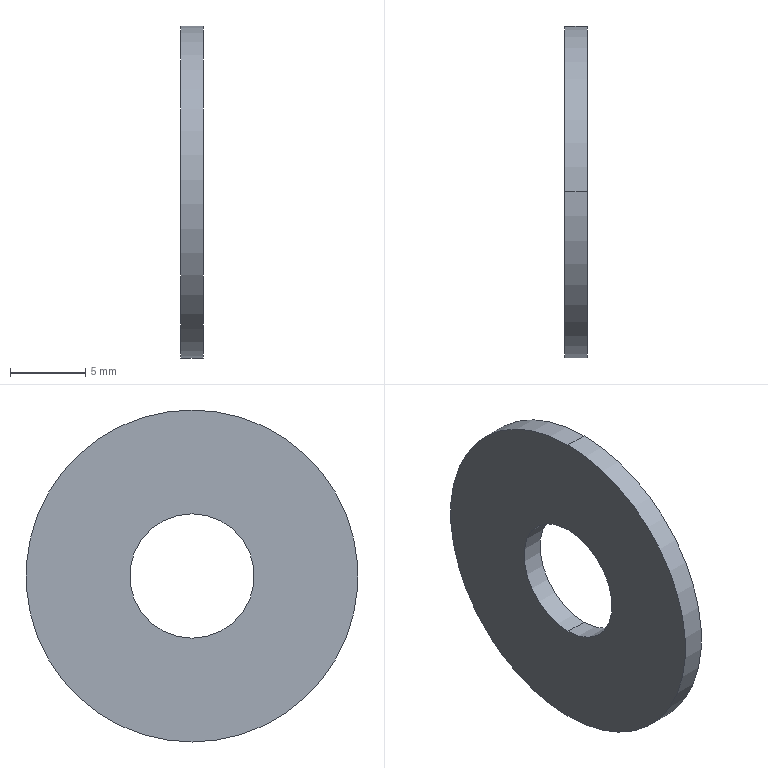Part | STEP file | 微波烘干-平输送机构-625058 | 1 solid | 6 faces | box 1.5 x 22 x 22 mm | volume 490.015 mm3 | cylinder 4 | plane 2 | commonest cylinder face diameters 8.25 x2 22 x2
STEP:
#1=CARTESIAN_POINT('',(1.5,0.,-4.125));
#2=VERTEX_POINT('',#1);
#3=CARTESIAN_POINT('',(1.5,0.,4.125));
#4=VERTEX_POINT('',#3);
#5=CARTESIAN_POINT('',(1.5,0.,0.));
#6=DIRECTION('',(-1.,0.,0.));
#7=DIRECTION('',(0.,0.,1.));
#8=AXIS2_PLACEMENT_3D('',#5,#6,#7);
#9=CIRCLE('',#8,4.125);
#10=EDGE_CURVE('',#2,#4,#9,.T.);
#11=ORIENTED_EDGE('',*,*,#10,.F.);
#12=CARTESIAN_POINT('',(0.,0.,-4.125));
#13=VERTEX_POINT('',#12);
#14=CARTESIAN_POINT('',(1.5,0.,-4.125));
#15=DIRECTION('',(-1.,0.,0.));
#16=VECTOR('',#15,1000.);
#17=LINE('',#14,#16);
#18=EDGE_CURVE('',#2,#13,#17,.T.);
#19=ORIENTED_EDGE('',*,*,#18,.T.);
#20=CARTESIAN_POINT('',(0.,0.,4.125));
#21=VERTEX_POINT('',#20);
#22=CARTESIAN_POINT('',(0.,0.,0.));
#23=DIRECTION('',(-1.,0.,0.));
#24=DIRECTION('',(0.,0.,1.));
#25=AXIS2_PLACEMENT_3D('',#22,#23,#24);
#26=CIRCLE('',#25,4.125);
#27=EDGE_CURVE('',#13,#21,#26,.T.);
#28=ORIENTED_EDGE('',*,*,#27,.T.);
#29=CARTESIAN_POINT('',(1.5,0.,4.125));
#30=DIRECTION('',(-1.,0.,0.));
#31=VECTOR('',#30,1000.);
#32=LINE('',#29,#31);
#33=EDGE_CURVE('',#4,#21,#32,.T.);
#34=ORIENTED_EDGE('',*,*,#33,.F.);
#35=EDGE_LOOP('',(#11,#19,#28,#34));
#36=FACE_OUTER_BOUND('',#35,.T.);
#37=CARTESIAN_POINT('',(1.5,0.,0.));
#38=DIRECTION('',(-1.,0.,0.));
#39=DIRECTION('',(0.,0.,1.));
#40=AXIS2_PLACEMENT_3D('',#37,#38,#39);
#41=CYLINDRICAL_SURFACE('',#40,4.125);
#42=ADVANCED_FACE('',(#36),#41,.F.);
#43=CARTESIAN_POINT('',(1.5,0.,-11.));
#44=VERTEX_POINT('',#43);
#45=CARTESIAN_POINT('',(1.5,0.,11.));
#46=VERTEX_POINT('',#45);
#47=CARTESIAN_POINT('',(1.5,0.,0.));
#48=DIRECTION('',(1.,0.,0.));
#49=DIRECTION('',(0.,0.,1.));
#50=AXIS2_PLACEMENT_3D('',#47,#48,#49);
#51=CIRCLE('',#50,11.);
#52=EDGE_CURVE('',#44,#46,#51,.T.);
#53=ORIENTED_EDGE('',*,*,#52,.F.);
#54=CARTESIAN_POINT('',(0.,0.,-11.));
#55=VERTEX_POINT('',#54);
#56=CARTESIAN_POINT('',(0.75,0.,-11.));
#57=DIRECTION('',(-1.,0.,0.));
#58=VECTOR('',#57,1000.);
#59=LINE('',#56,#58);
#60=EDGE_CURVE('',#44,#55,#59,.T.);
#61=ORIENTED_EDGE('',*,*,#60,.T.);
#62=CARTESIAN_POINT('',(0.,0.,11.));
#63=VERTEX_POINT('',#62);
#64=CARTESIAN_POINT('',(0.,0.,0.));
#65=DIRECTION('',(1.,0.,0.));
#66=DIRECTION('',(0.,0.,1.));
#67=AXIS2_PLACEMENT_3D('',#64,#65,#66);
#68=CIRCLE('',#67,11.);
#69=EDGE_CURVE('',#55,#63,#68,.T.);
#70=ORIENTED_EDGE('',*,*,#69,.T.);
#71=CARTESIAN_POINT('',(0.75,0.,11.));
#72=DIRECTION('',(-1.,0.,0.));
#73=VECTOR('',#72,1000.);
#74=LINE('',#71,#73);
#75=EDGE_CURVE('',#46,#63,#74,.T.);
#76=ORIENTED_EDGE('',*,*,#75,.F.);
#77=EDGE_LOOP('',(#53,#61,#70,#76));
#78=FACE_OUTER_BOUND('',#77,.T.);
#79=CARTESIAN_POINT('',(0.75,0.,0.));
#80=DIRECTION('',(-1.,0.,0.));
#81=DIRECTION('',(0.,0.,1.));
#82=AXIS2_PLACEMENT_3D('',#79,#80,#81);
#83=CYLINDRICAL_SURFACE('',#82,11.);
#84=ADVANCED_FACE('',(#78),#83,.T.);
#85=CARTESIAN_POINT('',(1.5,0.,0.));
#86=DIRECTION('',(-1.,0.,0.));
#87=DIRECTION('',(0.,0.,1.));
#88=AXIS2_PLACEMENT_3D('',#85,#86,#87);
#89=CIRCLE('',#88,4.125);
#90=EDGE_CURVE('',#4,#2,#89,.T.);
#91=ORIENTED_EDGE('',*,*,#90,.T.);
#92=ORIENTED_EDGE('',*,*,#10,.T.);
#93=EDGE_LOOP('',(#91,#92));
#94=FACE_BOUND('',#93,.T.);
#95=CARTESIAN_POINT('',(1.5,0.,0.));
#96=DIRECTION('',(1.,0.,0.));
#97=DIRECTION('',(0.,0.,1.));
#98=AXIS2_PLACEMENT_3D('',#95,#96,#97);
#99=CIRCLE('',#98,11.);
#100=EDGE_CURVE('',#46,#44,#99,.T.);
#101=ORIENTED_EDGE('',*,*,#100,.T.);
#102=ORIENTED_EDGE('',*,*,#52,.T.);
#103=EDGE_LOOP('',(#101,#102));
#104=FACE_OUTER_BOUND('',#103,.T.);
#105=CARTESIAN_POINT('',(1.5,0.,-7.562));
#106=DIRECTION('',(1.,0.,0.));
#107=DIRECTION('',(0.,0.,-1.));
#108=AXIS2_PLACEMENT_3D('',#105,#106,#107);
#109=PLANE('',#108);
#110=ADVANCED_FACE('',(#94,#104),#109,.T.);
#111=ORIENTED_EDGE('',*,*,#18,.F.);
#112=ORIENTED_EDGE('',*,*,#90,.F.);
#113=ORIENTED_EDGE('',*,*,#33,.T.);
#114=CARTESIAN_POINT('',(0.,0.,0.));
#115=DIRECTION('',(-1.,0.,0.));
#116=DIRECTION('',(0.,0.,1.));
#117=AXIS2_PLACEMENT_3D('',#114,#115,#116);
#118=CIRCLE('',#117,4.125);
#119=EDGE_CURVE('',#21,#13,#118,.T.);
#120=ORIENTED_EDGE('',*,*,#119,.T.);
#121=EDGE_LOOP('',(#111,#112,#113,#120));
#122=FACE_OUTER_BOUND('',#121,.T.);
#123=CARTESIAN_POINT('',(1.5,0.,0.));
#124=DIRECTION('',(-1.,0.,0.));
#125=DIRECTION('',(0.,0.,1.));
#126=AXIS2_PLACEMENT_3D('',#123,#124,#125);
#127=CYLINDRICAL_SURFACE('',#126,4.125);
#128=ADVANCED_FACE('',(#122),#127,.F.);
#129=ORIENTED_EDGE('',*,*,#60,.F.);
#130=ORIENTED_EDGE('',*,*,#100,.F.);
#131=ORIENTED_EDGE('',*,*,#75,.T.);
#132=CARTESIAN_POINT('',(0.,0.,0.));
#133=DIRECTION('',(1.,0.,0.));
#134=DIRECTION('',(0.,0.,1.));
#135=AXIS2_PLACEMENT_3D('',#132,#133,#134);
#136=CIRCLE('',#135,11.);
#137=EDGE_CURVE('',#63,#55,#136,.T.);
#138=ORIENTED_EDGE('',*,*,#137,.T.);
#139=EDGE_LOOP('',(#129,#130,#131,#138));
#140=FACE_OUTER_BOUND('',#139,.T.);
#141=CARTESIAN_POINT('',(0.75,0.,0.));
#142=DIRECTION('',(-1.,0.,0.));
#143=DIRECTION('',(0.,0.,1.));
#144=AXIS2_PLACEMENT_3D('',#141,#142,#143);
#145=CYLINDRICAL_SURFACE('',#144,11.);
#146=ADVANCED_FACE('',(#140),#145,.T.);
#147=ORIENTED_EDGE('',*,*,#137,.F.);
#148=ORIENTED_EDGE('',*,*,#69,.F.);
#149=EDGE_LOOP('',(#147,#148));
#150=FACE_OUTER_BOUND('',#149,.T.);
#151=ORIENTED_EDGE('',*,*,#119,.F.);
#152=ORIENTED_EDGE('',*,*,#27,.F.);
#153=EDGE_LOOP('',(#151,#152));
#154=FACE_BOUND('',#153,.T.);
#155=CARTESIAN_POINT('',(0.,0.,-7.562));
#156=DIRECTION('',(-1.,0.,0.));
#157=DIRECTION('',(0.,0.,1.));
#158=AXIS2_PLACEMENT_3D('',#155,#156,#157);
#159=PLANE('',#158);
#160=ADVANCED_FACE('',(#150,#154),#159,.T.);
#161=CLOSED_SHELL('',(#42,#84,#110,#128,#146,#160));
#162=MANIFOLD_SOLID_BREP('',#161);
#163=CARTESIAN_POINT('',(0.,0.,0.));
#164=DIRECTION('',(0.,0.,1.));
#165=DIRECTION('',(1.,0.,0.));
#166=AXIS2_PLACEMENT_3D('',#163,#164,#165);
#167=(LENGTH_UNIT()NAMED_UNIT(*)SI_UNIT(.MILLI.,.METRE.));
#168=UNCERTAINTY_MEASURE_WITH_UNIT(LENGTH_MEASURE(0.00001),#167,'','');
#169=(NAMED_UNIT(*)PLANE_ANGLE_UNIT()SI_UNIT($,.RADIAN.));
#170=(NAMED_UNIT(*)SI_UNIT($,.STERADIAN.)SOLID_ANGLE_UNIT());
#171=(GEOMETRIC_REPRESENTATION_CONTEXT(3)GLOBAL_UNCERTAINTY_ASSIGNED_CONTEXT((#168))GLOBAL_UNIT_ASSIGNED_CONTEXT((#167,#169,#170))REPRESENTATION_CONTEXT('',''));
#172=ADVANCED_BREP_SHAPE_REPRESENTATION('',(#162,#166),#171);